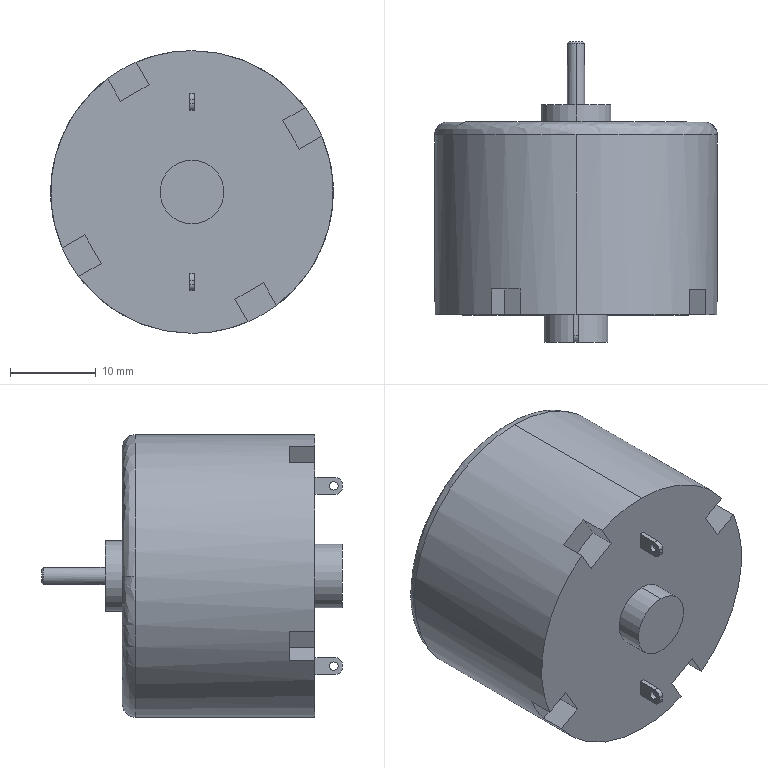Part | SolidWorks | features MoveFace 3, BaseBody 1, CirPattern 1, HoleWzd 1 | 1 solid | 75 faces | box 33 x 35.1 x 33 mm | volume 19096 mm3 | plane 31 | cylinder 28 | cone 14 | spline 2 | commonest cylinder face diameters 2.5 x12 1 x4 1.5 x4 2 x2 7.45 x2 8.2 x2